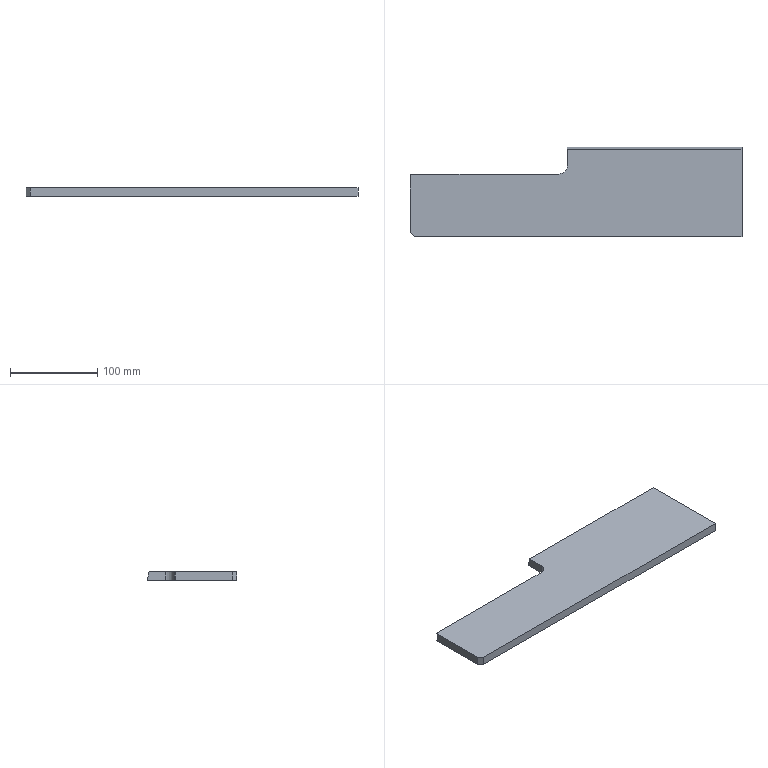Part | STEP file | 001-004-Feeding mechanism shaft slideway rear plate | 1 solid | 11 faces | box 380 x 102.993 x 10 mm | volume 333174 mm3 | plane 9 | cylinder 2 | commonest cylinder face diameters 4 x1 20 x1
STEP:
#1=CARTESIAN_POINT('',(0.,0.,0.));
#2=DIRECTION('',(0.,0.,1.));
#3=DIRECTION('',(1.,0.,0.));
#4=AXIS2_PLACEMENT_3D('',#1,#2,#3);
#5=CARTESIAN_POINT('',(190.,-50.25,0.));
#6=VERTEX_POINT('',#5);
#7=CARTESIAN_POINT('',(190.,52.743,0.));
#8=VERTEX_POINT('',#7);
#9=CARTESIAN_POINT('',(190.,-50.25,0.));
#10=DIRECTION('',(0.,1.,0.));
#11=VECTOR('',#10,1.);
#12=LINE('',#9,#11);
#13=CARTESIAN_POINT('',(190.,-50.25,10.));
#14=DIRECTION('',(-1.,0.,0.));
#15=DIRECTION('',(0.,0.,1.));
#16=AXIS2_PLACEMENT_3D('',#13,#14,#15);
#17=PLANE('',#16);
#18=CARTESIAN_POINT('',(-10.,0.));
#19=DIRECTION('',(0.,1.));
#20=VECTOR('',#19,1.);
#21=LINE('',#18,#20);
#22=(GEOMETRIC_REPRESENTATION_CONTEXT(2)PARAMETRIC_REPRESENTATION_CONTEXT()REPRESENTATION_CONTEXT('',''));
#23=DEFINITIONAL_REPRESENTATION('',(#21),#22);
#24=PCURVE('',#17,#23);
#25=CARTESIAN_POINT('',(0.,0.,0.));
#26=DIRECTION('',(0.,0.,-1.));
#27=DIRECTION('',(-1.,0.,0.));
#28=AXIS2_PLACEMENT_3D('',#25,#26,#27);
#29=PLANE('',#28);
#30=CARTESIAN_POINT('',(-190.,-50.25));
#31=DIRECTION('',(0.,1.));
#32=VECTOR('',#31,1.);
#33=LINE('',#30,#32);
#34=(GEOMETRIC_REPRESENTATION_CONTEXT(2)PARAMETRIC_REPRESENTATION_CONTEXT()REPRESENTATION_CONTEXT('',''));
#35=DEFINITIONAL_REPRESENTATION('',(#33),#34);
#36=PCURVE('',#29,#35);
#37=SURFACE_CURVE('',#12,(#24,#36),.PCURVE_S1.);
#38=EDGE_CURVE('',#6,#8,#37,.T.);
#39=ORIENTED_EDGE('',*,*,#38,.T.);
#40=CARTESIAN_POINT('',(190.,50.25,10.));
#41=VERTEX_POINT('',#40);
#42=CARTESIAN_POINT('',(190.,52.743,0.));
#43=DIRECTION('',(0.,-0.2419,0.9703));
#44=VECTOR('',#43,1.);
#45=LINE('',#42,#44);
#46=CARTESIAN_POINT('',(-10.,102.993));
#47=DIRECTION('',(0.9703,-0.2419));
#48=VECTOR('',#47,1.);
#49=LINE('',#46,#48);
#50=(GEOMETRIC_REPRESENTATION_CONTEXT(2)PARAMETRIC_REPRESENTATION_CONTEXT()REPRESENTATION_CONTEXT('',''));
#51=DEFINITIONAL_REPRESENTATION('',(#49),#50);
#52=PCURVE('',#17,#51);
#53=CARTESIAN_POINT('',(-190.,52.743,0.));
#54=DIRECTION('',(0.,0.9703,0.2419));
#55=DIRECTION('',(0.,-0.2419,0.9703));
#56=AXIS2_PLACEMENT_3D('',#53,#54,#55);
#57=PLANE('',#56);
#58=CARTESIAN_POINT('',(0.,380.));
#59=DIRECTION('',(1.,0.));
#60=VECTOR('',#59,1.);
#61=LINE('',#58,#60);
#62=(GEOMETRIC_REPRESENTATION_CONTEXT(2)PARAMETRIC_REPRESENTATION_CONTEXT()REPRESENTATION_CONTEXT('',''));
#63=DEFINITIONAL_REPRESENTATION('',(#61),#62);
#64=PCURVE('',#57,#63);
#65=SURFACE_CURVE('',#45,(#52,#64),.PCURVE_S1.);
#66=EDGE_CURVE('',#8,#41,#65,.T.);
#67=ORIENTED_EDGE('',*,*,#66,.T.);
#68=CARTESIAN_POINT('',(190.,-50.25,10.));
#69=VERTEX_POINT('',#68);
#70=CARTESIAN_POINT('',(190.,-50.25,10.));
#71=DIRECTION('',(0.,1.,0.));
#72=VECTOR('',#71,1.);
#73=LINE('',#70,#72);
#74=CARTESIAN_POINT('',(0.,0.));
#75=DIRECTION('',(0.,1.));
#76=VECTOR('',#75,1.);
#77=LINE('',#74,#76);
#78=(GEOMETRIC_REPRESENTATION_CONTEXT(2)PARAMETRIC_REPRESENTATION_CONTEXT()REPRESENTATION_CONTEXT('',''));
#79=DEFINITIONAL_REPRESENTATION('',(#77),#78);
#80=PCURVE('',#17,#79);
#81=CARTESIAN_POINT('',(0.,0.,10.));
#82=DIRECTION('',(0.,0.,-1.));
#83=DIRECTION('',(-1.,0.,0.));
#84=AXIS2_PLACEMENT_3D('',#81,#82,#83);
#85=PLANE('',#84);
#86=CARTESIAN_POINT('',(-190.,-50.25));
#87=DIRECTION('',(0.,1.));
#88=VECTOR('',#87,1.);
#89=LINE('',#86,#88);
#90=(GEOMETRIC_REPRESENTATION_CONTEXT(2)PARAMETRIC_REPRESENTATION_CONTEXT()REPRESENTATION_CONTEXT('',''));
#91=DEFINITIONAL_REPRESENTATION('',(#89),#90);
#92=PCURVE('',#85,#91);
#93=SURFACE_CURVE('',#73,(#80,#92),.PCURVE_S1.);
#94=EDGE_CURVE('',#69,#41,#93,.T.);
#95=ORIENTED_EDGE('',*,*,#94,.F.);
#96=CARTESIAN_POINT('',(190.,-50.25,10.));
#97=DIRECTION('',(0.,0.,-1.));
#98=VECTOR('',#97,1.);
#99=LINE('',#96,#98);
#100=CARTESIAN_POINT('',(0.,0.));
#101=DIRECTION('',(-1.,0.));
#102=VECTOR('',#101,1.);
#103=LINE('',#100,#102);
#104=(GEOMETRIC_REPRESENTATION_CONTEXT(2)PARAMETRIC_REPRESENTATION_CONTEXT()REPRESENTATION_CONTEXT('',''));
#105=DEFINITIONAL_REPRESENTATION('',(#103),#104);
#106=PCURVE('',#17,#105);
#107=CARTESIAN_POINT('',(-190.,-50.25,10.));
#108=DIRECTION('',(0.,1.,0.));
#109=DIRECTION('',(0.,0.,1.));
#110=AXIS2_PLACEMENT_3D('',#107,#108,#109);
#111=PLANE('',#110);
#112=CARTESIAN_POINT('',(0.,380.));
#113=DIRECTION('',(-1.,0.));
#114=VECTOR('',#113,1.);
#115=LINE('',#112,#114);
#116=(GEOMETRIC_REPRESENTATION_CONTEXT(2)PARAMETRIC_REPRESENTATION_CONTEXT()REPRESENTATION_CONTEXT('',''));
#117=DEFINITIONAL_REPRESENTATION('',(#115),#116);
#118=PCURVE('',#111,#117);
#119=SURFACE_CURVE('',#99,(#106,#118),.PCURVE_S1.);
#120=EDGE_CURVE('',#69,#6,#119,.T.);
#121=ORIENTED_EDGE('',*,*,#120,.T.);
#122=EDGE_LOOP('',(#39,#67,#95,#121));
#123=FACE_BOUND('',#122,.T.);
#124=ADVANCED_FACE('',(#123),#17,.F.);
#125=CARTESIAN_POINT('',(-190.,19.75,10.));
#126=VERTEX_POINT('',#125);
#127=CARTESIAN_POINT('',(-190.,-45.25,10.));
#128=VERTEX_POINT('',#127);
#129=CARTESIAN_POINT('',(-190.,-50.25,10.));
#130=DIRECTION('',(0.,-1.,0.));
#131=VECTOR('',#130,1.);
#132=LINE('',#129,#131);
#133=CARTESIAN_POINT('',(-190.,-50.25,10.));
#134=DIRECTION('',(1.,0.,0.));
#135=DIRECTION('',(0.,0.,-1.));
#136=AXIS2_PLACEMENT_3D('',#133,#134,#135);
#137=PLANE('',#136);
#138=CARTESIAN_POINT('',(0.,0.));
#139=DIRECTION('',(0.,-1.));
#140=VECTOR('',#139,1.);
#141=LINE('',#138,#140);
#142=(GEOMETRIC_REPRESENTATION_CONTEXT(2)PARAMETRIC_REPRESENTATION_CONTEXT()REPRESENTATION_CONTEXT('',''));
#143=DEFINITIONAL_REPRESENTATION('',(#141),#142);
#144=PCURVE('',#137,#143);
#145=CARTESIAN_POINT('',(190.,-50.25));
#146=DIRECTION('',(0.,-1.));
#147=VECTOR('',#146,1.);
#148=LINE('',#145,#147);
#149=(GEOMETRIC_REPRESENTATION_CONTEXT(2)PARAMETRIC_REPRESENTATION_CONTEXT()REPRESENTATION_CONTEXT('',''));
#150=DEFINITIONAL_REPRESENTATION('',(#148),#149);
#151=PCURVE('',#85,#150);
#152=SURFACE_CURVE('',#132,(#144,#151),.PCURVE_S1.);
#153=EDGE_CURVE('',#126,#128,#152,.T.);
#154=ORIENTED_EDGE('',*,*,#153,.F.);
#155=CARTESIAN_POINT('',(-190.,19.75,0.));
#156=VERTEX_POINT('',#155);
#157=CARTESIAN_POINT('',(-190.,19.75,10.));
#158=DIRECTION('',(0.,0.,-1.));
#159=VECTOR('',#158,1.);
#160=LINE('',#157,#159);
#161=CARTESIAN_POINT('',(0.,70.));
#162=DIRECTION('',(1.,0.));
#163=VECTOR('',#162,1.);
#164=LINE('',#161,#163);
#165=(GEOMETRIC_REPRESENTATION_CONTEXT(2)PARAMETRIC_REPRESENTATION_CONTEXT()REPRESENTATION_CONTEXT('',''));
#166=DEFINITIONAL_REPRESENTATION('',(#164),#165);
#167=PCURVE('',#137,#166);
#168=CARTESIAN_POINT('',(-188.,19.75,10.));
#169=DIRECTION('',(0.,0.,-1.));
#170=DIRECTION('',(-1.,0.,0.));
#171=AXIS2_PLACEMENT_3D('',#168,#169,#170);
#172=CYLINDRICAL_SURFACE('',#171,2.);
#173=CARTESIAN_POINT('',(0.,0.));
#174=DIRECTION('',(0.,1.));
#175=VECTOR('',#174,1.);
#176=LINE('',#173,#175);
#177=(GEOMETRIC_REPRESENTATION_CONTEXT(2)PARAMETRIC_REPRESENTATION_CONTEXT()REPRESENTATION_CONTEXT('',''));
#178=DEFINITIONAL_REPRESENTATION('',(#176),#177);
#179=PCURVE('',#172,#178);
#180=SURFACE_CURVE('',#160,(#167,#179),.PCURVE_S1.);
#181=EDGE_CURVE('',#126,#156,#180,.T.);
#182=ORIENTED_EDGE('',*,*,#181,.T.);
#183=CARTESIAN_POINT('',(-190.,-45.25,0.));
#184=VERTEX_POINT('',#183);
#185=CARTESIAN_POINT('',(-190.,-50.25,0.));
#186=DIRECTION('',(0.,-1.,0.));
#187=VECTOR('',#186,1.);
#188=LINE('',#185,#187);
#189=CARTESIAN_POINT('',(10.,0.));
#190=DIRECTION('',(0.,-1.));
#191=VECTOR('',#190,1.);
#192=LINE('',#189,#191);
#193=(GEOMETRIC_REPRESENTATION_CONTEXT(2)PARAMETRIC_REPRESENTATION_CONTEXT()REPRESENTATION_CONTEXT('',''));
#194=DEFINITIONAL_REPRESENTATION('',(#192),#193);
#195=PCURVE('',#137,#194);
#196=CARTESIAN_POINT('',(190.,-50.25));
#197=DIRECTION('',(0.,-1.));
#198=VECTOR('',#197,1.);
#199=LINE('',#196,#198);
#200=(GEOMETRIC_REPRESENTATION_CONTEXT(2)PARAMETRIC_REPRESENTATION_CONTEXT()REPRESENTATION_CONTEXT('',''));
#201=DEFINITIONAL_REPRESENTATION('',(#199),#200);
#202=PCURVE('',#29,#201);
#203=SURFACE_CURVE('',#188,(#195,#202),.PCURVE_S1.);
#204=EDGE_CURVE('',#156,#184,#203,.T.);
#205=ORIENTED_EDGE('',*,*,#204,.T.);
#206=CARTESIAN_POINT('',(-190.,-45.25,10.));
#207=DIRECTION('',(0.,0.,1.));
#208=VECTOR('',#207,1.);
#209=LINE('',#206,#208);
#210=CARTESIAN_POINT('',(0.,5.));
#211=DIRECTION('',(-1.,0.));
#212=VECTOR('',#211,1.);
#213=LINE('',#210,#212);
#214=(GEOMETRIC_REPRESENTATION_CONTEXT(2)PARAMETRIC_REPRESENTATION_CONTEXT()REPRESENTATION_CONTEXT('',''));
#215=DEFINITIONAL_REPRESENTATION('',(#213),#214);
#216=PCURVE('',#137,#215);
#217=CARTESIAN_POINT('',(-185.,-50.25,10.));
#218=DIRECTION('',(0.7071,0.7071,0.));
#219=DIRECTION('',(0.,0.,-1.));
#220=AXIS2_PLACEMENT_3D('',#217,#218,#219);
#221=PLANE('',#220);
#222=CARTESIAN_POINT('',(0.,7.071));
#223=DIRECTION('',(-1.,0.));
#224=VECTOR('',#223,1.);
#225=LINE('',#222,#224);
#226=(GEOMETRIC_REPRESENTATION_CONTEXT(2)PARAMETRIC_REPRESENTATION_CONTEXT()REPRESENTATION_CONTEXT('',''));
#227=DEFINITIONAL_REPRESENTATION('',(#225),#226);
#228=PCURVE('',#221,#227);
#229=SURFACE_CURVE('',#209,(#216,#228),.PCURVE_S1.);
#230=EDGE_CURVE('',#184,#128,#229,.T.);
#231=ORIENTED_EDGE('',*,*,#230,.T.);
#232=EDGE_LOOP('',(#154,#182,#205,#231));
#233=FACE_BOUND('',#232,.T.);
#234=ADVANCED_FACE('',(#233),#137,.F.);
#235=CARTESIAN_POINT('',(-185.,-50.25,10.));
#236=VERTEX_POINT('',#235);
#237=CARTESIAN_POINT('',(-190.,-50.25,10.));
#238=DIRECTION('',(1.,0.,0.));
#239=VECTOR('',#238,1.);
#240=LINE('',#237,#239);
#241=CARTESIAN_POINT('',(0.,0.));
#242=DIRECTION('',(0.,1.));
#243=VECTOR('',#242,1.);
#244=LINE('',#241,#243);
#245=(GEOMETRIC_REPRESENTATION_CONTEXT(2)PARAMETRIC_REPRESENTATION_CONTEXT()REPRESENTATION_CONTEXT('',''));
#246=DEFINITIONAL_REPRESENTATION('',(#244),#245);
#247=PCURVE('',#111,#246);
#248=CARTESIAN_POINT('',(190.,-50.25));
#249=DIRECTION('',(-1.,0.));
#250=VECTOR('',#249,1.);
#251=LINE('',#248,#250);
#252=(GEOMETRIC_REPRESENTATION_CONTEXT(2)PARAMETRIC_REPRESENTATION_CONTEXT()REPRESENTATION_CONTEXT('',''));
#253=DEFINITIONAL_REPRESENTATION('',(#251),#252);
#254=PCURVE('',#85,#253);
#255=SURFACE_CURVE('',#240,(#247,#254),.PCURVE_S1.);
#256=EDGE_CURVE('',#236,#69,#255,.T.);
#257=ORIENTED_EDGE('',*,*,#256,.F.);
#258=CARTESIAN_POINT('',(-185.,-50.25,0.));
#259=VERTEX_POINT('',#258);
#260=CARTESIAN_POINT('',(-185.,-50.25,10.));
#261=DIRECTION('',(0.,0.,-1.));
#262=VECTOR('',#261,1.);
#263=LINE('',#260,#262);
#264=CARTESIAN_POINT('',(0.,5.));
#265=DIRECTION('',(-1.,0.));
#266=VECTOR('',#265,1.);
#267=LINE('',#264,#266);
#268=(GEOMETRIC_REPRESENTATION_CONTEXT(2)PARAMETRIC_REPRESENTATION_CONTEXT()REPRESENTATION_CONTEXT('',''));
#269=DEFINITIONAL_REPRESENTATION('',(#267),#268);
#270=PCURVE('',#111,#269);
#271=CARTESIAN_POINT('',(0.,0.));
#272=DIRECTION('',(1.,0.));
#273=VECTOR('',#272,1.);
#274=LINE('',#271,#273);
#275=(GEOMETRIC_REPRESENTATION_CONTEXT(2)PARAMETRIC_REPRESENTATION_CONTEXT()REPRESENTATION_CONTEXT('',''));
#276=DEFINITIONAL_REPRESENTATION('',(#274),#275);
#277=PCURVE('',#221,#276);
#278=SURFACE_CURVE('',#263,(#270,#277),.PCURVE_S1.);
#279=EDGE_CURVE('',#236,#259,#278,.T.);
#280=ORIENTED_EDGE('',*,*,#279,.T.);
#281=CARTESIAN_POINT('',(-190.,-50.25,0.));
#282=DIRECTION('',(1.,0.,0.));
#283=VECTOR('',#282,1.);
#284=LINE('',#281,#283);
#285=CARTESIAN_POINT('',(-10.,0.));
#286=DIRECTION('',(0.,1.));
#287=VECTOR('',#286,1.);
#288=LINE('',#285,#287);
#289=(GEOMETRIC_REPRESENTATION_CONTEXT(2)PARAMETRIC_REPRESENTATION_CONTEXT()REPRESENTATION_CONTEXT('',''));
#290=DEFINITIONAL_REPRESENTATION('',(#288),#289);
#291=PCURVE('',#111,#290);
#292=CARTESIAN_POINT('',(190.,-50.25));
#293=DIRECTION('',(-1.,0.));
#294=VECTOR('',#293,1.);
#295=LINE('',#292,#294);
#296=(GEOMETRIC_REPRESENTATION_CONTEXT(2)PARAMETRIC_REPRESENTATION_CONTEXT()REPRESENTATION_CONTEXT('',''));
#297=DEFINITIONAL_REPRESENTATION('',(#295),#296);
#298=PCURVE('',#29,#297);
#299=SURFACE_CURVE('',#284,(#291,#298),.PCURVE_S1.);
#300=EDGE_CURVE('',#259,#6,#299,.T.);
#301=ORIENTED_EDGE('',*,*,#300,.T.);
#302=ORIENTED_EDGE('',*,*,#120,.F.);
#303=EDGE_LOOP('',(#257,#280,#301,#302));
#304=FACE_BOUND('',#303,.T.);
#305=ADVANCED_FACE('',(#304),#111,.F.);
#306=CARTESIAN_POINT('',(-20.,21.75,10.));
#307=VERTEX_POINT('',#306);
#308=CARTESIAN_POINT('',(-188.,21.75,10.));
#309=VERTEX_POINT('',#308);
#310=CARTESIAN_POINT('',(-190.,21.75,10.));
#311=DIRECTION('',(-1.,0.,0.));
#312=VECTOR('',#311,1.);
#313=LINE('',#310,#312);
#314=CARTESIAN_POINT('',(190.,21.75));
#315=DIRECTION('',(1.,0.));
#316=VECTOR('',#315,1.);
#317=LINE('',#314,#316);
#318=(GEOMETRIC_REPRESENTATION_CONTEXT(2)PARAMETRIC_REPRESENTATION_CONTEXT()REPRESENTATION_CONTEXT('',''));
#319=DEFINITIONAL_REPRESENTATION('',(#317),#318);
#320=PCURVE('',#85,#319);
#321=CARTESIAN_POINT('',(-190.,21.75,10.));
#322=DIRECTION('',(0.,-1.,0.));
#323=DIRECTION('',(1.,0.,0.));
#324=AXIS2_PLACEMENT_3D('',#321,#322,#323);
#325=PLANE('',#324);
#326=CARTESIAN_POINT('',(0.,0.));
#327=DIRECTION('',(-1.,0.));
#328=VECTOR('',#327,1.);
#329=LINE('',#326,#328);
#330=(GEOMETRIC_REPRESENTATION_CONTEXT(2)PARAMETRIC_REPRESENTATION_CONTEXT()REPRESENTATION_CONTEXT('',''));
#331=DEFINITIONAL_REPRESENTATION('',(#329),#330);
#332=PCURVE('',#325,#331);
#333=SURFACE_CURVE('',#313,(#320,#332),.PCURVE_S1.);
#334=EDGE_CURVE('',#307,#309,#333,.T.);
#335=ORIENTED_EDGE('',*,*,#334,.T.);
#336=CARTESIAN_POINT('',(-188.,19.75,10.));
#337=DIRECTION('',(0.,0.,1.));
#338=DIRECTION('',(-1.,0.,0.));
#339=AXIS2_PLACEMENT_3D('',#336,#337,#338);
#340=CIRCLE('',#339,2.);
#341=CARTESIAN_POINT('',(190.,19.75));
#342=CARTESIAN_POINT('',(190.,16.286));
#343=CARTESIAN_POINT('',(187.,18.018));
#344=CARTESIAN_POINT('',(184.,19.75));
#345=CARTESIAN_POINT('',(187.,21.482));
#346=CARTESIAN_POINT('',(190.,23.214));
#347=CARTESIAN_POINT('',(190.,19.75));
#348=(BOUNDED_CURVE()B_SPLINE_CURVE(2,(#341,#342,#343,#344,#345,#346,#347),.UNSPECIFIED.,.T.,.F.)B_SPLINE_CURVE_WITH_KNOTS((1,2,2,2,2,1),(-2.094,0.,2.094,4.189,6.283,8.378),.UNSPECIFIED.)CURVE()GEOMETRIC_REPRESENTATION_ITEM()RATIONAL_B_SPLINE_CURVE((1.,0.5,1.,0.5,1.,0.5,1.))REPRESENTATION_ITEM(''));
#349=(GEOMETRIC_REPRESENTATION_CONTEXT(2)PARAMETRIC_REPRESENTATION_CONTEXT()REPRESENTATION_CONTEXT('',''));
#350=DEFINITIONAL_REPRESENTATION('',(#348),#349);
#351=PCURVE('',#85,#350);
#352=CARTESIAN_POINT('',(6.283,0.));
#353=DIRECTION('',(-1.,0.));
#354=VECTOR('',#353,1.);
#355=LINE('',#352,#354);
#356=(GEOMETRIC_REPRESENTATION_CONTEXT(2)PARAMETRIC_REPRESENTATION_CONTEXT()REPRESENTATION_CONTEXT('',''));
#357=DEFINITIONAL_REPRESENTATION('',(#355),#356);
#358=PCURVE('',#172,#357);
#359=SURFACE_CURVE('',#340,(#351,#358),.PCURVE_S1.);
#360=EDGE_CURVE('',#309,#126,#359,.T.);
#361=ORIENTED_EDGE('',*,*,#360,.T.);
#362=ORIENTED_EDGE('',*,*,#153,.T.);
#363=CARTESIAN_POINT('',(-185.,-50.25,10.));
#364=DIRECTION('',(0.7071,-0.7071,0.));
#365=VECTOR('',#364,1.);
#366=LINE('',#363,#365);
#367=CARTESIAN_POINT('',(185.,-50.25));
#368=DIRECTION('',(-0.7071,-0.7071));
#369=VECTOR('',#368,1.);
#370=LINE('',#367,#369);
#371=(GEOMETRIC_REPRESENTATION_CONTEXT(2)PARAMETRIC_REPRESENTATION_CONTEXT()REPRESENTATION_CONTEXT('',''));
#372=DEFINITIONAL_REPRESENTATION('',(#370),#371);
#373=PCURVE('',#85,#372);
#374=CARTESIAN_POINT('',(0.,0.));
#375=DIRECTION('',(0.,-1.));
#376=VECTOR('',#375,1.);
#377=LINE('',#374,#376);
#378=(GEOMETRIC_REPRESENTATION_CONTEXT(2)PARAMETRIC_REPRESENTATION_CONTEXT()REPRESENTATION_CONTEXT('',''));
#379=DEFINITIONAL_REPRESENTATION('',(#377),#378);
#380=PCURVE('',#221,#379);
#381=SURFACE_CURVE('',#366,(#373,#380),.PCURVE_S1.);
#382=EDGE_CURVE('',#128,#236,#381,.T.);
#383=ORIENTED_EDGE('',*,*,#382,.T.);
#384=ORIENTED_EDGE('',*,*,#256,.T.);
#385=ORIENTED_EDGE('',*,*,#94,.T.);
#386=CARTESIAN_POINT('',(-10.,50.25,10.));
#387=VERTEX_POINT('',#386);
#388=CARTESIAN_POINT('',(-190.,50.25,10.));
#389=DIRECTION('',(-1.,0.,0.));
#390=VECTOR('',#389,1.);
#391=LINE('',#388,#390);
#392=CARTESIAN_POINT('',(190.,50.25));
#393=DIRECTION('',(1.,0.));
#394=VECTOR('',#393,1.);
#395=LINE('',#392,#394);
#396=(GEOMETRIC_REPRESENTATION_CONTEXT(2)PARAMETRIC_REPRESENTATION_CONTEXT()REPRESENTATION_CONTEXT('',''));
#397=DEFINITIONAL_REPRESENTATION('',(#395),#396);
#398=PCURVE('',#85,#397);
#399=CARTESIAN_POINT('',(10.306,0.));
#400=DIRECTION('',(0.,-1.));
#401=VECTOR('',#400,1.);
#402=LINE('',#399,#401);
#403=(GEOMETRIC_REPRESENTATION_CONTEXT(2)PARAMETRIC_REPRESENTATION_CONTEXT()REPRESENTATION_CONTEXT('',''));
#404=DEFINITIONAL_REPRESENTATION('',(#402),#403);
#405=PCURVE('',#57,#404);
#406=SURFACE_CURVE('',#391,(#398,#405),.PCURVE_S1.);
#407=EDGE_CURVE('',#41,#387,#406,.T.);
#408=ORIENTED_EDGE('',*,*,#407,.T.);
#409=CARTESIAN_POINT('',(-10.,31.75,10.));
#410=VERTEX_POINT('',#409);
#411=CARTESIAN_POINT('',(-10.,52.743,10.));
#412=DIRECTION('',(0.,-1.,0.));
#413=VECTOR('',#412,1.);
#414=LINE('',#411,#413);
#415=CARTESIAN_POINT('',(10.,52.743));
#416=DIRECTION('',(0.,-1.));
#417=VECTOR('',#416,1.);
#418=LINE('',#415,#417);
#419=(GEOMETRIC_REPRESENTATION_CONTEXT(2)PARAMETRIC_REPRESENTATION_CONTEXT()REPRESENTATION_CONTEXT('',''));
#420=DEFINITIONAL_REPRESENTATION('',(#418),#419);
#421=PCURVE('',#85,#420);
#422=CARTESIAN_POINT('',(-10.,52.743,10.));
#423=DIRECTION('',(1.,0.,0.));
#424=DIRECTION('',(0.,1.,0.));
#425=AXIS2_PLACEMENT_3D('',#422,#423,#424);
#426=PLANE('',#425);
#427=CARTESIAN_POINT('',(0.,0.));
#428=DIRECTION('',(-1.,0.));
#429=VECTOR('',#428,1.);
#430=LINE('',#427,#429);
#431=(GEOMETRIC_REPRESENTATION_CONTEXT(2)PARAMETRIC_REPRESENTATION_CONTEXT()REPRESENTATION_CONTEXT('',''));
#432=DEFINITIONAL_REPRESENTATION('',(#430),#431);
#433=PCURVE('',#426,#432);
#434=SURFACE_CURVE('',#414,(#421,#433),.PCURVE_S1.);
#435=EDGE_CURVE('',#387,#410,#434,.T.);
#436=ORIENTED_EDGE('',*,*,#435,.T.);
#437=CARTESIAN_POINT('',(-20.,31.75,10.));
#438=DIRECTION('',(0.,0.,-1.));
#439=DIRECTION('',(-1.,0.,0.));
#440=AXIS2_PLACEMENT_3D('',#437,#438,#439);
#441=CIRCLE('',#440,10.);
#442=CARTESIAN_POINT('',(20.,31.75));
#443=DIRECTION('',(1.,0.));
#444=AXIS2_PLACEMENT_2D('',#442,#443);
#445=CIRCLE('',#444,10.);
#446=(GEOMETRIC_REPRESENTATION_CONTEXT(2)PARAMETRIC_REPRESENTATION_CONTEXT()REPRESENTATION_CONTEXT('',''));
#447=DEFINITIONAL_REPRESENTATION('',(#445),#446);
#448=PCURVE('',#85,#447);
#449=CARTESIAN_POINT('',(-20.,31.75,10.));
#450=DIRECTION('',(0.,0.,1.));
#451=DIRECTION('',(1.,0.,0.));
#452=AXIS2_PLACEMENT_3D('',#449,#450,#451);
#453=CYLINDRICAL_SURFACE('',#452,10.);
#454=CARTESIAN_POINT('',(9.425,0.));
#455=DIRECTION('',(-1.,0.));
#456=VECTOR('',#455,1.);
#457=LINE('',#454,#456);
#458=(GEOMETRIC_REPRESENTATION_CONTEXT(2)PARAMETRIC_REPRESENTATION_CONTEXT()REPRESENTATION_CONTEXT('',''));
#459=DEFINITIONAL_REPRESENTATION('',(#457),#458);
#460=PCURVE('',#453,#459);
#461=SURFACE_CURVE('',#441,(#448,#460),.PCURVE_S1.);
#462=EDGE_CURVE('',#410,#307,#461,.T.);
#463=ORIENTED_EDGE('',*,*,#462,.T.);
#464=EDGE_LOOP('',(#335,#361,#362,#383,#384,#385,#408,#436,#463));
#465=FACE_BOUND('',#464,.T.);
#466=ADVANCED_FACE('',(#465),#85,.F.);
#467=ORIENTED_EDGE('',*,*,#204,.F.);
#468=CARTESIAN_POINT('',(-188.,21.75,0.));
#469=VERTEX_POINT('',#468);
#470=CARTESIAN_POINT('',(-188.,19.75,0.));
#471=DIRECTION('',(0.,0.,-1.));
#472=DIRECTION('',(-1.,0.,0.));
#473=AXIS2_PLACEMENT_3D('',#470,#471,#472);
#474=CIRCLE('',#473,2.);
#475=CARTESIAN_POINT('',(188.,19.75));
#476=DIRECTION('',(1.,0.));
#477=AXIS2_PLACEMENT_2D('',#475,#476);
#478=CIRCLE('',#477,2.);
#479=(GEOMETRIC_REPRESENTATION_CONTEXT(2)PARAMETRIC_REPRESENTATION_CONTEXT()REPRESENTATION_CONTEXT('',''));
#480=DEFINITIONAL_REPRESENTATION('',(#478),#479);
#481=PCURVE('',#29,#480);
#482=CARTESIAN_POINT('',(0.,10.));
#483=DIRECTION('',(1.,0.));
#484=VECTOR('',#483,1.);
#485=LINE('',#482,#484);
#486=(GEOMETRIC_REPRESENTATION_CONTEXT(2)PARAMETRIC_REPRESENTATION_CONTEXT()REPRESENTATION_CONTEXT('',''));
#487=DEFINITIONAL_REPRESENTATION('',(#485),#486);
#488=PCURVE('',#172,#487);
#489=SURFACE_CURVE('',#474,(#481,#488),.PCURVE_S1.);
#490=EDGE_CURVE('',#156,#469,#489,.T.);
#491=ORIENTED_EDGE('',*,*,#490,.T.);
#492=CARTESIAN_POINT('',(-20.,21.75,0.));
#493=VERTEX_POINT('',#492);
#494=CARTESIAN_POINT('',(-190.,21.75,0.));
#495=DIRECTION('',(-1.,0.,0.));
#496=VECTOR('',#495,1.);
#497=LINE('',#494,#496);
#498=CARTESIAN_POINT('',(190.,21.75));
#499=DIRECTION('',(1.,0.));
#500=VECTOR('',#499,1.);
#501=LINE('',#498,#500);
#502=(GEOMETRIC_REPRESENTATION_CONTEXT(2)PARAMETRIC_REPRESENTATION_CONTEXT()REPRESENTATION_CONTEXT('',''));
#503=DEFINITIONAL_REPRESENTATION('',(#501),#502);
#504=PCURVE('',#29,#503);
#505=CARTESIAN_POINT('',(0.,-10.));
#506=DIRECTION('',(-1.,0.));
#507=VECTOR('',#506,1.);
#508=LINE('',#505,#507);
#509=(GEOMETRIC_REPRESENTATION_CONTEXT(2)PARAMETRIC_REPRESENTATION_CONTEXT()REPRESENTATION_CONTEXT('',''));
#510=DEFINITIONAL_REPRESENTATION('',(#508),#509);
#511=PCURVE('',#325,#510);
#512=SURFACE_CURVE('',#497,(#504,#511),.PCURVE_S1.);
#513=EDGE_CURVE('',#493,#469,#512,.T.);
#514=ORIENTED_EDGE('',*,*,#513,.F.);
#515=CARTESIAN_POINT('',(-10.,31.75,0.));
#516=VERTEX_POINT('',#515);
#517=CARTESIAN_POINT('',(-20.,31.75,0.));
#518=DIRECTION('',(0.,0.,1.));
#519=DIRECTION('',(-1.,0.,0.));
#520=AXIS2_PLACEMENT_3D('',#517,#518,#519);
#521=CIRCLE('',#520,10.);
#522=CARTESIAN_POINT('',(30.,31.75));
#523=CARTESIAN_POINT('',(30.,14.429));
#524=CARTESIAN_POINT('',(15.,23.09));
#525=CARTESIAN_POINT('',(0.,31.75));
#526=CARTESIAN_POINT('',(15.,40.41));
#527=CARTESIAN_POINT('',(30.,49.071));
#528=CARTESIAN_POINT('',(30.,31.75));
#529=(BOUNDED_CURVE()B_SPLINE_CURVE(2,(#522,#523,#524,#525,#526,#527,#528),.UNSPECIFIED.,.T.,.F.)B_SPLINE_CURVE_WITH_KNOTS((1,2,2,2,2,1),(-2.094,0.,2.094,4.189,6.283,8.378),.UNSPECIFIED.)CURVE()GEOMETRIC_REPRESENTATION_ITEM()RATIONAL_B_SPLINE_CURVE((1.,0.5,1.,0.5,1.,0.5,1.))REPRESENTATION_ITEM(''));
#530=(GEOMETRIC_REPRESENTATION_CONTEXT(2)PARAMETRIC_REPRESENTATION_CONTEXT()REPRESENTATION_CONTEXT('',''));
#531=DEFINITIONAL_REPRESENTATION('',(#529),#530);
#532=PCURVE('',#29,#531);
#533=CARTESIAN_POINT('',(3.142,-10.));
#534=DIRECTION('',(1.,0.));
#535=VECTOR('',#534,1.);
#536=LINE('',#533,#535);
#537=(GEOMETRIC_REPRESENTATION_CONTEXT(2)PARAMETRIC_REPRESENTATION_CONTEXT()REPRESENTATION_CONTEXT('',''));
#538=DEFINITIONAL_REPRESENTATION('',(#536),#537);
#539=PCURVE('',#453,#538);
#540=SURFACE_CURVE('',#521,(#532,#539),.PCURVE_S1.);
#541=EDGE_CURVE('',#493,#516,#540,.T.);
#542=ORIENTED_EDGE('',*,*,#541,.T.);
#543=CARTESIAN_POINT('',(-10.,52.743,0.));
#544=VERTEX_POINT('',#543);
#545=CARTESIAN_POINT('',(-10.,52.743,0.));
#546=DIRECTION('',(0.,-1.,0.));
#547=VECTOR('',#546,1.);
#548=LINE('',#545,#547);
#549=CARTESIAN_POINT('',(10.,52.743));
#550=DIRECTION('',(0.,-1.));
#551=VECTOR('',#550,1.);
#552=LINE('',#549,#551);
#553=(GEOMETRIC_REPRESENTATION_CONTEXT(2)PARAMETRIC_REPRESENTATION_CONTEXT()REPRESENTATION_CONTEXT('',''));
#554=DEFINITIONAL_REPRESENTATION('',(#552),#553);
#555=PCURVE('',#29,#554);
#556=CARTESIAN_POINT('',(0.,-10.));
#557=DIRECTION('',(-1.,0.));
#558=VECTOR('',#557,1.);
#559=LINE('',#556,#558);
#560=(GEOMETRIC_REPRESENTATION_CONTEXT(2)PARAMETRIC_REPRESENTATION_CONTEXT()REPRESENTATION_CONTEXT('',''));
#561=DEFINITIONAL_REPRESENTATION('',(#559),#560);
#562=PCURVE('',#426,#561);
#563=SURFACE_CURVE('',#548,(#555,#562),.PCURVE_S1.);
#564=EDGE_CURVE('',#544,#516,#563,.T.);
#565=ORIENTED_EDGE('',*,*,#564,.F.);
#566=CARTESIAN_POINT('',(-190.,52.743,0.));
#567=DIRECTION('',(1.,0.,0.));
#568=VECTOR('',#567,1.);
#569=LINE('',#566,#568);
#570=CARTESIAN_POINT('',(190.,52.743));
#571=DIRECTION('',(-1.,0.));
#572=VECTOR('',#571,1.);
#573=LINE('',#570,#572);
#574=(GEOMETRIC_REPRESENTATION_CONTEXT(2)PARAMETRIC_REPRESENTATION_CONTEXT()REPRESENTATION_CONTEXT('',''));
#575=DEFINITIONAL_REPRESENTATION('',(#573),#574);
#576=PCURVE('',#29,#575);
#577=CARTESIAN_POINT('',(0.,0.));
#578=DIRECTION('',(0.,1.));
#579=VECTOR('',#578,1.);
#580=LINE('',#577,#579);
#581=(GEOMETRIC_REPRESENTATION_CONTEXT(2)PARAMETRIC_REPRESENTATION_CONTEXT()REPRESENTATION_CONTEXT('',''));
#582=DEFINITIONAL_REPRESENTATION('',(#580),#581);
#583=PCURVE('',#57,#582);
#584=SURFACE_CURVE('',#569,(#576,#583),.PCURVE_S1.);
#585=EDGE_CURVE('',#544,#8,#584,.T.);
#586=ORIENTED_EDGE('',*,*,#585,.T.);
#587=ORIENTED_EDGE('',*,*,#38,.F.);
#588=ORIENTED_EDGE('',*,*,#300,.F.);
#589=CARTESIAN_POINT('',(-117.625,-117.625,0.));
#590=DIRECTION('',(-0.7071,0.7071,0.));
#591=VECTOR('',#590,1.);
#592=LINE('',#589,#591);
#593=CARTESIAN_POINT('',(117.625,-117.625));
#594=DIRECTION('',(0.7071,0.7071));
#595=VECTOR('',#594,1.);
#596=LINE('',#593,#595);
#597=(GEOMETRIC_REPRESENTATION_CONTEXT(2)PARAMETRIC_REPRESENTATION_CONTEXT()REPRESENTATION_CONTEXT('',''));
#598=DEFINITIONAL_REPRESENTATION('',(#596),#597);
#599=PCURVE('',#29,#598);
#600=CARTESIAN_POINT('',(10.,-95.283));
#601=DIRECTION('',(0.,1.));
#602=VECTOR('',#601,1.);
#603=LINE('',#600,#602);
#604=(GEOMETRIC_REPRESENTATION_CONTEXT(2)PARAMETRIC_REPRESENTATION_CONTEXT()REPRESENTATION_CONTEXT('',''));
#605=DEFINITIONAL_REPRESENTATION('',(#603),#604);
#606=PCURVE('',#221,#605);
#607=SURFACE_CURVE('',#592,(#599,#606),.PCURVE_S1.);
#608=EDGE_CURVE('',#259,#184,#607,.T.);
#609=ORIENTED_EDGE('',*,*,#608,.T.);
#610=EDGE_LOOP('',(#467,#491,#514,#542,#565,#586,#587,#588,#609));
#611=FACE_BOUND('',#610,.T.);
#612=ADVANCED_FACE('',(#611),#29,.T.);
#613=CARTESIAN_POINT('',(-10.,52.743,0.));
#614=DIRECTION('',(0.,0.2419,-0.9703));
#615=VECTOR('',#614,1.);
#616=LINE('',#613,#615);
#617=CARTESIAN_POINT('',(0.,180.));
#618=DIRECTION('',(-1.,0.));
#619=VECTOR('',#618,1.);
#620=LINE('',#617,#619);
#621=(GEOMETRIC_REPRESENTATION_CONTEXT(2)PARAMETRIC_REPRESENTATION_CONTEXT()REPRESENTATION_CONTEXT('',''));
#622=DEFINITIONAL_REPRESENTATION('',(#620),#621);
#623=PCURVE('',#57,#622);
#624=CARTESIAN_POINT('',(0.,-10.));
#625=DIRECTION('',(0.2419,-0.9703));
#626=VECTOR('',#625,1.);
#627=LINE('',#624,#626);
#628=(GEOMETRIC_REPRESENTATION_CONTEXT(2)PARAMETRIC_REPRESENTATION_CONTEXT()REPRESENTATION_CONTEXT('',''));
#629=DEFINITIONAL_REPRESENTATION('',(#627),#628);
#630=PCURVE('',#426,#629);
#631=SURFACE_CURVE('',#616,(#623,#630),.PCURVE_S1.);
#632=EDGE_CURVE('',#387,#544,#631,.T.);
#633=ORIENTED_EDGE('',*,*,#632,.F.);
#634=ORIENTED_EDGE('',*,*,#407,.F.);
#635=ORIENTED_EDGE('',*,*,#66,.F.);
#636=ORIENTED_EDGE('',*,*,#585,.F.);
#637=EDGE_LOOP('',(#633,#634,#635,#636));
#638=FACE_BOUND('',#637,.T.);
#639=ADVANCED_FACE('',(#638),#57,.T.);
#640=ORIENTED_EDGE('',*,*,#513,.T.);
#641=CARTESIAN_POINT('',(-188.,21.75,10.));
#642=DIRECTION('',(0.,0.,1.));
#643=VECTOR('',#642,1.);
#644=LINE('',#641,#643);
#645=CARTESIAN_POINT('',(2.,0.));
#646=DIRECTION('',(0.,1.));
#647=VECTOR('',#646,1.);
#648=LINE('',#645,#647);
#649=(GEOMETRIC_REPRESENTATION_CONTEXT(2)PARAMETRIC_REPRESENTATION_CONTEXT()REPRESENTATION_CONTEXT('',''));
#650=DEFINITIONAL_REPRESENTATION('',(#648),#649);
#651=PCURVE('',#325,#650);
#652=CARTESIAN_POINT('',(1.571,0.));
#653=DIRECTION('',(0.,-1.));
#654=VECTOR('',#653,1.);
#655=LINE('',#652,#654);
#656=(GEOMETRIC_REPRESENTATION_CONTEXT(2)PARAMETRIC_REPRESENTATION_CONTEXT()REPRESENTATION_CONTEXT('',''));
#657=DEFINITIONAL_REPRESENTATION('',(#655),#656);
#658=PCURVE('',#172,#657);
#659=SURFACE_CURVE('',#644,(#651,#658),.PCURVE_S1.);
#660=EDGE_CURVE('',#469,#309,#659,.T.);
#661=ORIENTED_EDGE('',*,*,#660,.T.);
#662=ORIENTED_EDGE('',*,*,#334,.F.);
#663=CARTESIAN_POINT('',(-20.,21.75,0.));
#664=DIRECTION('',(0.,0.,-1.));
#665=VECTOR('',#664,1.);
#666=LINE('',#663,#665);
#667=CARTESIAN_POINT('',(170.,-10.));
#668=DIRECTION('',(0.,-1.));
#669=VECTOR('',#668,1.);
#670=LINE('',#667,#669);
#671=(GEOMETRIC_REPRESENTATION_CONTEXT(2)PARAMETRIC_REPRESENTATION_CONTEXT()REPRESENTATION_CONTEXT('',''));
#672=DEFINITIONAL_REPRESENTATION('',(#670),#671);
#673=PCURVE('',#325,#672);
#674=CARTESIAN_POINT('',(4.712,-10.));
#675=DIRECTION('',(0.,-1.));
#676=VECTOR('',#675,1.);
#677=LINE('',#674,#676);
#678=(GEOMETRIC_REPRESENTATION_CONTEXT(2)PARAMETRIC_REPRESENTATION_CONTEXT()REPRESENTATION_CONTEXT('',''));
#679=DEFINITIONAL_REPRESENTATION('',(#677),#678);
#680=PCURVE('',#453,#679);
#681=SURFACE_CURVE('',#666,(#673,#680),.PCURVE_S1.);
#682=EDGE_CURVE('',#307,#493,#681,.T.);
#683=ORIENTED_EDGE('',*,*,#682,.T.);
#684=EDGE_LOOP('',(#640,#661,#662,#683));
#685=FACE_BOUND('',#684,.T.);
#686=ADVANCED_FACE('',(#685),#325,.F.);
#687=ORIENTED_EDGE('',*,*,#564,.T.);
#688=CARTESIAN_POINT('',(-10.,31.75,10.));
#689=DIRECTION('',(0.,0.,1.));
#690=VECTOR('',#689,1.);
#691=LINE('',#688,#690);
#692=CARTESIAN_POINT('',(-20.993,0.));
#693=DIRECTION('',(0.,1.));
#694=VECTOR('',#693,1.);
#695=LINE('',#692,#694);
#696=(GEOMETRIC_REPRESENTATION_CONTEXT(2)PARAMETRIC_REPRESENTATION_CONTEXT()REPRESENTATION_CONTEXT('',''));
#697=DEFINITIONAL_REPRESENTATION('',(#695),#696);
#698=PCURVE('',#426,#697);
#699=CARTESIAN_POINT('',(6.283,0.));
#700=DIRECTION('',(0.,1.));
#701=VECTOR('',#700,1.);
#702=LINE('',#699,#701);
#703=(GEOMETRIC_REPRESENTATION_CONTEXT(2)PARAMETRIC_REPRESENTATION_CONTEXT()REPRESENTATION_CONTEXT('',''));
#704=DEFINITIONAL_REPRESENTATION('',(#702),#703);
#705=PCURVE('',#453,#704);
#706=SURFACE_CURVE('',#691,(#698,#705),.PCURVE_S1.);
#707=EDGE_CURVE('',#516,#410,#706,.T.);
#708=ORIENTED_EDGE('',*,*,#707,.T.);
#709=ORIENTED_EDGE('',*,*,#435,.F.);
#710=ORIENTED_EDGE('',*,*,#632,.T.);
#711=EDGE_LOOP('',(#687,#708,#709,#710));
#712=FACE_BOUND('',#711,.T.);
#713=ADVANCED_FACE('',(#712),#426,.F.);
#714=ORIENTED_EDGE('',*,*,#682,.T.);
#715=ORIENTED_EDGE('',*,*,#541,.T.);
#716=ORIENTED_EDGE('',*,*,#707,.T.);
#717=ORIENTED_EDGE('',*,*,#462,.T.);
#718=EDGE_LOOP('',(#714,#715,#716,#717));
#719=FACE_BOUND('',#718,.F.);
#720=ADVANCED_FACE('',(#719),#453,.F.);
#721=ORIENTED_EDGE('',*,*,#382,.F.);
#722=ORIENTED_EDGE('',*,*,#230,.F.);
#723=ORIENTED_EDGE('',*,*,#608,.F.);
#724=ORIENTED_EDGE('',*,*,#279,.F.);
#725=EDGE_LOOP('',(#721,#722,#723,#724));
#726=FACE_BOUND('',#725,.T.);
#727=ADVANCED_FACE('',(#726),#221,.F.);
#728=ORIENTED_EDGE('',*,*,#360,.F.);
#729=ORIENTED_EDGE('',*,*,#660,.F.);
#730=ORIENTED_EDGE('',*,*,#490,.F.);
#731=ORIENTED_EDGE('',*,*,#181,.F.);
#732=EDGE_LOOP('',(#728,#729,#730,#731));
#733=FACE_BOUND('',#732,.T.);
#734=ADVANCED_FACE('',(#733),#172,.T.);
#735=CLOSED_SHELL('',(#124,#234,#305,#466,#612,#639,#686,#713,#720,#727,#734));
#736=MANIFOLD_SOLID_BREP('',#735);
#737=(LENGTH_UNIT()NAMED_UNIT(*)SI_UNIT(.MILLI.,.METRE.));
#738=UNCERTAINTY_MEASURE_WITH_UNIT(LENGTH_MEASURE(0.0000001),#737,'','');
#739=(NAMED_UNIT(*)PLANE_ANGLE_UNIT()SI_UNIT($,.RADIAN.));
#740=(NAMED_UNIT(*)SI_UNIT($,.STERADIAN.)SOLID_ANGLE_UNIT());
#741=(GEOMETRIC_REPRESENTATION_CONTEXT(3)GLOBAL_UNCERTAINTY_ASSIGNED_CONTEXT((#738))GLOBAL_UNIT_ASSIGNED_CONTEXT((#737,#739,#740))REPRESENTATION_CONTEXT('',''));
#742=ADVANCED_BREP_SHAPE_REPRESENTATION('',(#4,#736),#741);